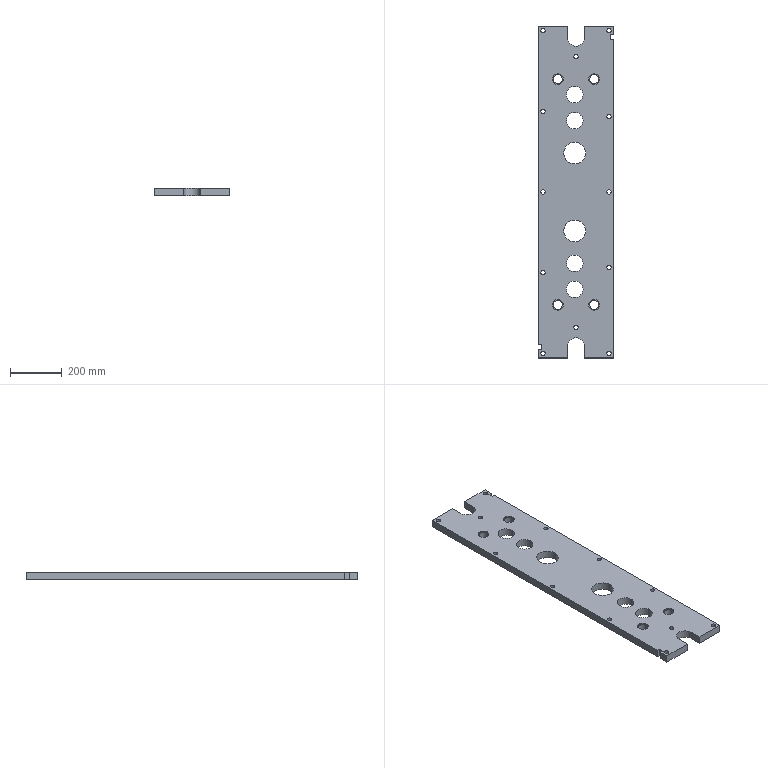Part | STEP file | 4-20.sldasm-Part-246 | 1 solid | 114 faces | box 290 x 1280 x 30 mm | volume 9865062 mm3 | cylinder 78 | plane 36 | commonest cylinder face diameters 16.667 x24 25.4 x24 34.938 x8 41.421 x8 64 x8 84 x4